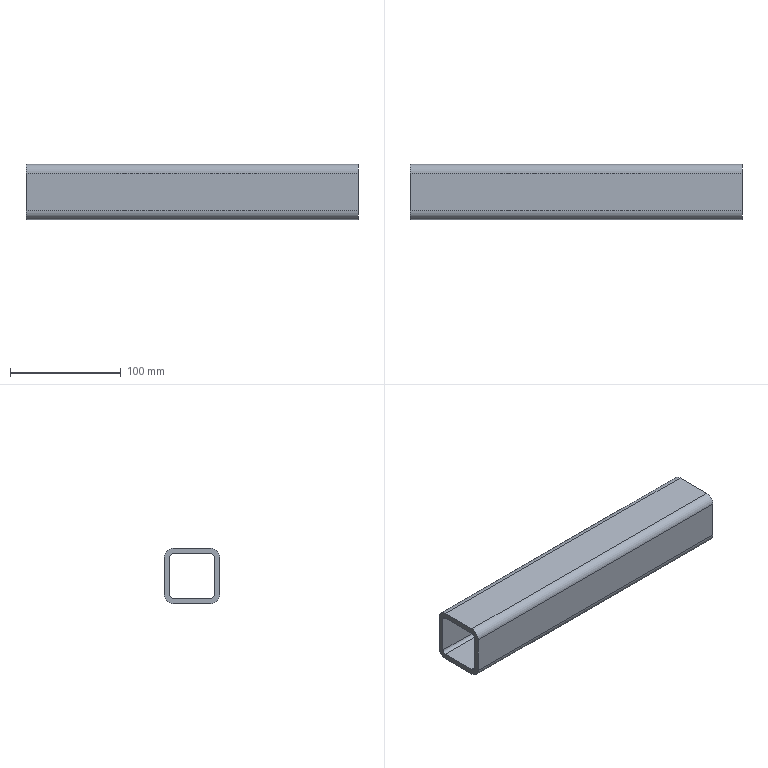Part | SolidWorks | features WeldMemberFeat 1, WeldmentFeature 1 | 1 solid | 18 faces | box 300 x 50 x 50 mm | volume 255836 mm3 | plane 10 | cylinder 8 | commonest cylinder face diameters 6 x4 16 x4
STEP:
#1=CARTESIAN_POINT('',(-88.434,25.,17.));
#2=VERTEX_POINT('',#1);
#3=CARTESIAN_POINT('',(-88.434,17.,25.));
#4=VERTEX_POINT('',#3);
#5=CARTESIAN_POINT('',(-88.434,17.,17.));
#6=DIRECTION('',(1.,0.,0.));
#7=DIRECTION('',(0.,0.,-1.));
#8=AXIS2_PLACEMENT_3D('',#5,#6,#7);
#9=CIRCLE('',#8,8.);
#10=EDGE_CURVE('',#2,#4,#9,.T.);
#11=ORIENTED_EDGE('',*,*,#10,.T.);
#12=CARTESIAN_POINT('',(211.566,17.,25.));
#13=VERTEX_POINT('',#12);
#14=CARTESIAN_POINT('',(211.566,17.,25.));
#15=DIRECTION('',(-1.,0.,0.));
#16=VECTOR('',#15,1000.);
#17=LINE('',#14,#16);
#18=EDGE_CURVE('',#13,#4,#17,.T.);
#19=ORIENTED_EDGE('',*,*,#18,.F.);
#20=CARTESIAN_POINT('',(211.566,25.,17.));
#21=VERTEX_POINT('',#20);
#22=CARTESIAN_POINT('',(211.566,17.,17.));
#23=DIRECTION('',(1.,0.,0.));
#24=DIRECTION('',(0.,0.,-1.));
#25=AXIS2_PLACEMENT_3D('',#22,#23,#24);
#26=CIRCLE('',#25,8.);
#27=EDGE_CURVE('',#21,#13,#26,.T.);
#28=ORIENTED_EDGE('',*,*,#27,.F.);
#29=CARTESIAN_POINT('',(211.566,25.,17.));
#30=DIRECTION('',(-1.,0.,0.));
#31=VECTOR('',#30,1000.);
#32=LINE('',#29,#31);
#33=EDGE_CURVE('',#21,#2,#32,.T.);
#34=ORIENTED_EDGE('',*,*,#33,.T.);
#35=EDGE_LOOP('',(#11,#19,#28,#34));
#36=FACE_OUTER_BOUND('',#35,.T.);
#37=CARTESIAN_POINT('',(211.566,17.,17.));
#38=DIRECTION('',(-1.,0.,0.));
#39=DIRECTION('',(0.,0.,1.));
#40=AXIS2_PLACEMENT_3D('',#37,#38,#39);
#41=CYLINDRICAL_SURFACE('',#40,8.);
#42=ADVANCED_FACE('',(#36),#41,.T.);
#43=CARTESIAN_POINT('',(-88.434,-17.,25.));
#44=VERTEX_POINT('',#43);
#45=CARTESIAN_POINT('',(-88.434,17.,25.));
#46=DIRECTION('',(0.,-1.,0.));
#47=VECTOR('',#46,1000.);
#48=LINE('',#45,#47);
#49=EDGE_CURVE('',#4,#44,#48,.T.);
#50=ORIENTED_EDGE('',*,*,#49,.T.);
#51=CARTESIAN_POINT('',(211.566,-17.,25.));
#52=VERTEX_POINT('',#51);
#53=CARTESIAN_POINT('',(211.566,-17.,25.));
#54=DIRECTION('',(-1.,0.,0.));
#55=VECTOR('',#54,1000.);
#56=LINE('',#53,#55);
#57=EDGE_CURVE('',#52,#44,#56,.T.);
#58=ORIENTED_EDGE('',*,*,#57,.F.);
#59=CARTESIAN_POINT('',(211.566,17.,25.));
#60=DIRECTION('',(0.,-1.,0.));
#61=VECTOR('',#60,1000.);
#62=LINE('',#59,#61);
#63=EDGE_CURVE('',#13,#52,#62,.T.);
#64=ORIENTED_EDGE('',*,*,#63,.F.);
#65=ORIENTED_EDGE('',*,*,#18,.T.);
#66=EDGE_LOOP('',(#50,#58,#64,#65));
#67=FACE_OUTER_BOUND('',#66,.T.);
#68=CARTESIAN_POINT('',(211.566,17.,25.));
#69=DIRECTION('',(0.,0.,-1.));
#70=DIRECTION('',(-1.,0.,0.));
#71=AXIS2_PLACEMENT_3D('',#68,#69,#70);
#72=PLANE('',#71);
#73=ADVANCED_FACE('',(#67),#72,.F.);
#74=CARTESIAN_POINT('',(-88.434,-25.,17.));
#75=VERTEX_POINT('',#74);
#76=CARTESIAN_POINT('',(-88.434,-17.,17.));
#77=DIRECTION('',(1.,0.,0.));
#78=DIRECTION('',(0.,0.,-1.));
#79=AXIS2_PLACEMENT_3D('',#76,#77,#78);
#80=CIRCLE('',#79,8.);
#81=EDGE_CURVE('',#44,#75,#80,.T.);
#82=ORIENTED_EDGE('',*,*,#81,.T.);
#83=CARTESIAN_POINT('',(211.566,-25.,17.));
#84=VERTEX_POINT('',#83);
#85=CARTESIAN_POINT('',(211.566,-25.,17.));
#86=DIRECTION('',(-1.,0.,0.));
#87=VECTOR('',#86,1000.);
#88=LINE('',#85,#87);
#89=EDGE_CURVE('',#84,#75,#88,.T.);
#90=ORIENTED_EDGE('',*,*,#89,.F.);
#91=CARTESIAN_POINT('',(211.566,-17.,17.));
#92=DIRECTION('',(1.,0.,0.));
#93=DIRECTION('',(0.,0.,-1.));
#94=AXIS2_PLACEMENT_3D('',#91,#92,#93);
#95=CIRCLE('',#94,8.);
#96=EDGE_CURVE('',#52,#84,#95,.T.);
#97=ORIENTED_EDGE('',*,*,#96,.F.);
#98=ORIENTED_EDGE('',*,*,#57,.T.);
#99=EDGE_LOOP('',(#82,#90,#97,#98));
#100=FACE_OUTER_BOUND('',#99,.T.);
#101=CARTESIAN_POINT('',(211.566,-17.,17.));
#102=DIRECTION('',(-1.,0.,0.));
#103=DIRECTION('',(0.,0.,1.));
#104=AXIS2_PLACEMENT_3D('',#101,#102,#103);
#105=CYLINDRICAL_SURFACE('',#104,8.);
#106=ADVANCED_FACE('',(#100),#105,.T.);
#107=CARTESIAN_POINT('',(-88.434,-25.,-17.));
#108=VERTEX_POINT('',#107);
#109=CARTESIAN_POINT('',(-88.434,-25.,-17.));
#110=DIRECTION('',(0.,0.,-1.));
#111=VECTOR('',#110,1000.);
#112=LINE('',#109,#111);
#113=EDGE_CURVE('',#75,#108,#112,.T.);
#114=ORIENTED_EDGE('',*,*,#113,.T.);
#115=CARTESIAN_POINT('',(211.566,-25.,-17.));
#116=VERTEX_POINT('',#115);
#117=CARTESIAN_POINT('',(211.566,-25.,-17.));
#118=DIRECTION('',(-1.,0.,0.));
#119=VECTOR('',#118,1000.);
#120=LINE('',#117,#119);
#121=EDGE_CURVE('',#116,#108,#120,.T.);
#122=ORIENTED_EDGE('',*,*,#121,.F.);
#123=CARTESIAN_POINT('',(211.566,-25.,-17.));
#124=DIRECTION('',(0.,0.,-1.));
#125=VECTOR('',#124,1000.);
#126=LINE('',#123,#125);
#127=EDGE_CURVE('',#84,#116,#126,.T.);
#128=ORIENTED_EDGE('',*,*,#127,.F.);
#129=ORIENTED_EDGE('',*,*,#89,.T.);
#130=EDGE_LOOP('',(#114,#122,#128,#129));
#131=FACE_OUTER_BOUND('',#130,.T.);
#132=CARTESIAN_POINT('',(211.566,-25.,-17.));
#133=DIRECTION('',(0.,1.,0.));
#134=DIRECTION('',(0.,0.,1.));
#135=AXIS2_PLACEMENT_3D('',#132,#133,#134);
#136=PLANE('',#135);
#137=ADVANCED_FACE('',(#131),#136,.F.);
#138=CARTESIAN_POINT('',(-88.434,-17.,-25.));
#139=VERTEX_POINT('',#138);
#140=CARTESIAN_POINT('',(-88.434,-17.,-17.));
#141=DIRECTION('',(1.,0.,0.));
#142=DIRECTION('',(0.,0.,-1.));
#143=AXIS2_PLACEMENT_3D('',#140,#141,#142);
#144=CIRCLE('',#143,8.);
#145=EDGE_CURVE('',#108,#139,#144,.T.);
#146=ORIENTED_EDGE('',*,*,#145,.T.);
#147=CARTESIAN_POINT('',(211.566,-17.,-25.));
#148=VERTEX_POINT('',#147);
#149=CARTESIAN_POINT('',(211.566,-17.,-25.));
#150=DIRECTION('',(-1.,0.,0.));
#151=VECTOR('',#150,1000.);
#152=LINE('',#149,#151);
#153=EDGE_CURVE('',#148,#139,#152,.T.);
#154=ORIENTED_EDGE('',*,*,#153,.F.);
#155=CARTESIAN_POINT('',(211.566,-17.,-17.));
#156=DIRECTION('',(1.,0.,0.));
#157=DIRECTION('',(0.,0.,-1.));
#158=AXIS2_PLACEMENT_3D('',#155,#156,#157);
#159=CIRCLE('',#158,8.);
#160=EDGE_CURVE('',#116,#148,#159,.T.);
#161=ORIENTED_EDGE('',*,*,#160,.F.);
#162=ORIENTED_EDGE('',*,*,#121,.T.);
#163=EDGE_LOOP('',(#146,#154,#161,#162));
#164=FACE_OUTER_BOUND('',#163,.T.);
#165=CARTESIAN_POINT('',(211.566,-17.,-17.));
#166=DIRECTION('',(-1.,0.,0.));
#167=DIRECTION('',(0.,0.,1.));
#168=AXIS2_PLACEMENT_3D('',#165,#166,#167);
#169=CYLINDRICAL_SURFACE('',#168,8.);
#170=ADVANCED_FACE('',(#164),#169,.T.);
#171=CARTESIAN_POINT('',(-88.434,17.,-25.));
#172=VERTEX_POINT('',#171);
#173=CARTESIAN_POINT('',(-88.434,-17.,-25.));
#174=DIRECTION('',(0.,1.,0.));
#175=VECTOR('',#174,1000.);
#176=LINE('',#173,#175);
#177=EDGE_CURVE('',#139,#172,#176,.T.);
#178=ORIENTED_EDGE('',*,*,#177,.T.);
#179=CARTESIAN_POINT('',(211.566,17.,-25.));
#180=VERTEX_POINT('',#179);
#181=CARTESIAN_POINT('',(211.566,17.,-25.));
#182=DIRECTION('',(-1.,0.,0.));
#183=VECTOR('',#182,1000.);
#184=LINE('',#181,#183);
#185=EDGE_CURVE('',#180,#172,#184,.T.);
#186=ORIENTED_EDGE('',*,*,#185,.F.);
#187=CARTESIAN_POINT('',(211.566,-17.,-25.));
#188=DIRECTION('',(0.,1.,0.));
#189=VECTOR('',#188,1000.);
#190=LINE('',#187,#189);
#191=EDGE_CURVE('',#148,#180,#190,.T.);
#192=ORIENTED_EDGE('',*,*,#191,.F.);
#193=ORIENTED_EDGE('',*,*,#153,.T.);
#194=EDGE_LOOP('',(#178,#186,#192,#193));
#195=FACE_OUTER_BOUND('',#194,.T.);
#196=CARTESIAN_POINT('',(211.566,-17.,-25.));
#197=DIRECTION('',(0.,0.,1.));
#198=DIRECTION('',(1.,0.,0.));
#199=AXIS2_PLACEMENT_3D('',#196,#197,#198);
#200=PLANE('',#199);
#201=ADVANCED_FACE('',(#195),#200,.F.);
#202=CARTESIAN_POINT('',(-88.434,25.,-17.));
#203=VERTEX_POINT('',#202);
#204=CARTESIAN_POINT('',(-88.434,17.,-17.));
#205=DIRECTION('',(1.,0.,0.));
#206=DIRECTION('',(0.,0.,-1.));
#207=AXIS2_PLACEMENT_3D('',#204,#205,#206);
#208=CIRCLE('',#207,8.);
#209=EDGE_CURVE('',#172,#203,#208,.T.);
#210=ORIENTED_EDGE('',*,*,#209,.T.);
#211=CARTESIAN_POINT('',(211.566,25.,-17.));
#212=VERTEX_POINT('',#211);
#213=CARTESIAN_POINT('',(211.566,25.,-17.));
#214=DIRECTION('',(-1.,0.,0.));
#215=VECTOR('',#214,1000.);
#216=LINE('',#213,#215);
#217=EDGE_CURVE('',#212,#203,#216,.T.);
#218=ORIENTED_EDGE('',*,*,#217,.F.);
#219=CARTESIAN_POINT('',(211.566,17.,-17.));
#220=DIRECTION('',(1.,0.,0.));
#221=DIRECTION('',(0.,0.,-1.));
#222=AXIS2_PLACEMENT_3D('',#219,#220,#221);
#223=CIRCLE('',#222,8.);
#224=EDGE_CURVE('',#180,#212,#223,.T.);
#225=ORIENTED_EDGE('',*,*,#224,.F.);
#226=ORIENTED_EDGE('',*,*,#185,.T.);
#227=EDGE_LOOP('',(#210,#218,#225,#226));
#228=FACE_OUTER_BOUND('',#227,.T.);
#229=CARTESIAN_POINT('',(211.566,17.,-17.));
#230=DIRECTION('',(-1.,0.,0.));
#231=DIRECTION('',(0.,0.,1.));
#232=AXIS2_PLACEMENT_3D('',#229,#230,#231);
#233=CYLINDRICAL_SURFACE('',#232,8.);
#234=ADVANCED_FACE('',(#228),#233,.T.);
#235=CARTESIAN_POINT('',(-88.434,-17.,20.));
#236=VERTEX_POINT('',#235);
#237=CARTESIAN_POINT('',(-88.434,-20.,17.));
#238=VERTEX_POINT('',#237);
#239=CARTESIAN_POINT('',(-88.434,-17.,17.));
#240=DIRECTION('',(1.,0.,0.));
#241=DIRECTION('',(0.,0.,-1.));
#242=AXIS2_PLACEMENT_3D('',#239,#240,#241);
#243=CIRCLE('',#242,3.);
#244=EDGE_CURVE('',#236,#238,#243,.T.);
#245=ORIENTED_EDGE('',*,*,#244,.F.);
#246=CARTESIAN_POINT('',(211.566,-17.,20.));
#247=VERTEX_POINT('',#246);
#248=CARTESIAN_POINT('',(211.566,-17.,20.));
#249=DIRECTION('',(-1.,0.,0.));
#250=VECTOR('',#249,1000.);
#251=LINE('',#248,#250);
#252=EDGE_CURVE('',#247,#236,#251,.T.);
#253=ORIENTED_EDGE('',*,*,#252,.F.);
#254=CARTESIAN_POINT('',(211.566,-20.,17.));
#255=VERTEX_POINT('',#254);
#256=CARTESIAN_POINT('',(211.566,-17.,17.));
#257=DIRECTION('',(1.,0.,0.));
#258=DIRECTION('',(0.,0.,-1.));
#259=AXIS2_PLACEMENT_3D('',#256,#257,#258);
#260=CIRCLE('',#259,3.);
#261=EDGE_CURVE('',#247,#255,#260,.T.);
#262=ORIENTED_EDGE('',*,*,#261,.T.);
#263=CARTESIAN_POINT('',(211.566,-20.,17.));
#264=DIRECTION('',(-1.,0.,0.));
#265=VECTOR('',#264,1000.);
#266=LINE('',#263,#265);
#267=EDGE_CURVE('',#255,#238,#266,.T.);
#268=ORIENTED_EDGE('',*,*,#267,.T.);
#269=EDGE_LOOP('',(#245,#253,#262,#268));
#270=FACE_OUTER_BOUND('',#269,.T.);
#271=CARTESIAN_POINT('',(211.566,-17.,17.));
#272=DIRECTION('',(-1.,0.,0.));
#273=DIRECTION('',(0.,0.,1.));
#274=AXIS2_PLACEMENT_3D('',#271,#272,#273);
#275=CYLINDRICAL_SURFACE('',#274,3.);
#276=ADVANCED_FACE('',(#270),#275,.F.);
#277=CARTESIAN_POINT('',(-88.434,17.,20.));
#278=VERTEX_POINT('',#277);
#279=CARTESIAN_POINT('',(-88.434,17.,20.));
#280=DIRECTION('',(0.,-1.,0.));
#281=VECTOR('',#280,1000.);
#282=LINE('',#279,#281);
#283=EDGE_CURVE('',#278,#236,#282,.T.);
#284=ORIENTED_EDGE('',*,*,#283,.F.);
#285=CARTESIAN_POINT('',(211.566,17.,20.));
#286=VERTEX_POINT('',#285);
#287=CARTESIAN_POINT('',(211.566,17.,20.));
#288=DIRECTION('',(-1.,0.,0.));
#289=VECTOR('',#288,1000.);
#290=LINE('',#287,#289);
#291=EDGE_CURVE('',#286,#278,#290,.T.);
#292=ORIENTED_EDGE('',*,*,#291,.F.);
#293=CARTESIAN_POINT('',(211.566,17.,20.));
#294=DIRECTION('',(0.,-1.,0.));
#295=VECTOR('',#294,1000.);
#296=LINE('',#293,#295);
#297=EDGE_CURVE('',#286,#247,#296,.T.);
#298=ORIENTED_EDGE('',*,*,#297,.T.);
#299=ORIENTED_EDGE('',*,*,#252,.T.);
#300=EDGE_LOOP('',(#284,#292,#298,#299));
#301=FACE_OUTER_BOUND('',#300,.T.);
#302=CARTESIAN_POINT('',(211.566,17.,20.));
#303=DIRECTION('',(0.,0.,-1.));
#304=DIRECTION('',(-1.,0.,0.));
#305=AXIS2_PLACEMENT_3D('',#302,#303,#304);
#306=PLANE('',#305);
#307=ADVANCED_FACE('',(#301),#306,.T.);
#308=CARTESIAN_POINT('',(-88.434,20.,17.));
#309=VERTEX_POINT('',#308);
#310=CARTESIAN_POINT('',(-88.434,17.,17.));
#311=DIRECTION('',(1.,0.,0.));
#312=DIRECTION('',(0.,0.,-1.));
#313=AXIS2_PLACEMENT_3D('',#310,#311,#312);
#314=CIRCLE('',#313,3.);
#315=EDGE_CURVE('',#309,#278,#314,.T.);
#316=ORIENTED_EDGE('',*,*,#315,.F.);
#317=CARTESIAN_POINT('',(211.566,20.,17.));
#318=VERTEX_POINT('',#317);
#319=CARTESIAN_POINT('',(211.566,20.,17.));
#320=DIRECTION('',(-1.,0.,0.));
#321=VECTOR('',#320,1000.);
#322=LINE('',#319,#321);
#323=EDGE_CURVE('',#318,#309,#322,.T.);
#324=ORIENTED_EDGE('',*,*,#323,.F.);
#325=CARTESIAN_POINT('',(211.566,17.,17.));
#326=DIRECTION('',(1.,0.,0.));
#327=DIRECTION('',(0.,0.,-1.));
#328=AXIS2_PLACEMENT_3D('',#325,#326,#327);
#329=CIRCLE('',#328,3.);
#330=EDGE_CURVE('',#318,#286,#329,.T.);
#331=ORIENTED_EDGE('',*,*,#330,.T.);
#332=ORIENTED_EDGE('',*,*,#291,.T.);
#333=EDGE_LOOP('',(#316,#324,#331,#332));
#334=FACE_OUTER_BOUND('',#333,.T.);
#335=CARTESIAN_POINT('',(211.566,17.,17.));
#336=DIRECTION('',(-1.,0.,0.));
#337=DIRECTION('',(0.,0.,1.));
#338=AXIS2_PLACEMENT_3D('',#335,#336,#337);
#339=CYLINDRICAL_SURFACE('',#338,3.);
#340=ADVANCED_FACE('',(#334),#339,.F.);
#341=CARTESIAN_POINT('',(-88.434,20.,-17.));
#342=VERTEX_POINT('',#341);
#343=CARTESIAN_POINT('',(-88.434,20.,17.));
#344=DIRECTION('',(0.,0.,1.));
#345=VECTOR('',#344,1000.);
#346=LINE('',#343,#345);
#347=EDGE_CURVE('',#342,#309,#346,.T.);
#348=ORIENTED_EDGE('',*,*,#347,.F.);
#349=CARTESIAN_POINT('',(211.566,20.,-17.));
#350=VERTEX_POINT('',#349);
#351=CARTESIAN_POINT('',(211.566,20.,-17.));
#352=DIRECTION('',(-1.,0.,0.));
#353=VECTOR('',#352,1000.);
#354=LINE('',#351,#353);
#355=EDGE_CURVE('',#350,#342,#354,.T.);
#356=ORIENTED_EDGE('',*,*,#355,.F.);
#357=CARTESIAN_POINT('',(211.566,20.,17.));
#358=DIRECTION('',(0.,0.,1.));
#359=VECTOR('',#358,1000.);
#360=LINE('',#357,#359);
#361=EDGE_CURVE('',#350,#318,#360,.T.);
#362=ORIENTED_EDGE('',*,*,#361,.T.);
#363=ORIENTED_EDGE('',*,*,#323,.T.);
#364=EDGE_LOOP('',(#348,#356,#362,#363));
#365=FACE_OUTER_BOUND('',#364,.T.);
#366=CARTESIAN_POINT('',(211.566,20.,17.));
#367=DIRECTION('',(0.,-1.,0.));
#368=DIRECTION('',(0.,0.,-1.));
#369=AXIS2_PLACEMENT_3D('',#366,#367,#368);
#370=PLANE('',#369);
#371=ADVANCED_FACE('',(#365),#370,.T.);
#372=CARTESIAN_POINT('',(-88.434,17.,-20.));
#373=VERTEX_POINT('',#372);
#374=CARTESIAN_POINT('',(-88.434,17.,-17.));
#375=DIRECTION('',(1.,0.,0.));
#376=DIRECTION('',(0.,0.,-1.));
#377=AXIS2_PLACEMENT_3D('',#374,#375,#376);
#378=CIRCLE('',#377,3.);
#379=EDGE_CURVE('',#373,#342,#378,.T.);
#380=ORIENTED_EDGE('',*,*,#379,.F.);
#381=CARTESIAN_POINT('',(211.566,17.,-20.));
#382=VERTEX_POINT('',#381);
#383=CARTESIAN_POINT('',(211.566,17.,-20.));
#384=DIRECTION('',(-1.,0.,0.));
#385=VECTOR('',#384,1000.);
#386=LINE('',#383,#385);
#387=EDGE_CURVE('',#382,#373,#386,.T.);
#388=ORIENTED_EDGE('',*,*,#387,.F.);
#389=CARTESIAN_POINT('',(211.566,17.,-17.));
#390=DIRECTION('',(1.,0.,0.));
#391=DIRECTION('',(0.,0.,-1.));
#392=AXIS2_PLACEMENT_3D('',#389,#390,#391);
#393=CIRCLE('',#392,3.);
#394=EDGE_CURVE('',#382,#350,#393,.T.);
#395=ORIENTED_EDGE('',*,*,#394,.T.);
#396=ORIENTED_EDGE('',*,*,#355,.T.);
#397=EDGE_LOOP('',(#380,#388,#395,#396));
#398=FACE_OUTER_BOUND('',#397,.T.);
#399=CARTESIAN_POINT('',(211.566,17.,-17.));
#400=DIRECTION('',(-1.,0.,0.));
#401=DIRECTION('',(0.,0.,1.));
#402=AXIS2_PLACEMENT_3D('',#399,#400,#401);
#403=CYLINDRICAL_SURFACE('',#402,3.);
#404=ADVANCED_FACE('',(#398),#403,.F.);
#405=CARTESIAN_POINT('',(-88.434,-17.,-20.));
#406=VERTEX_POINT('',#405);
#407=CARTESIAN_POINT('',(-88.434,-17.,-20.));
#408=DIRECTION('',(0.,1.,0.));
#409=VECTOR('',#408,1000.);
#410=LINE('',#407,#409);
#411=EDGE_CURVE('',#406,#373,#410,.T.);
#412=ORIENTED_EDGE('',*,*,#411,.F.);
#413=CARTESIAN_POINT('',(211.566,-17.,-20.));
#414=VERTEX_POINT('',#413);
#415=CARTESIAN_POINT('',(211.566,-17.,-20.));
#416=DIRECTION('',(-1.,0.,0.));
#417=VECTOR('',#416,1000.);
#418=LINE('',#415,#417);
#419=EDGE_CURVE('',#414,#406,#418,.T.);
#420=ORIENTED_EDGE('',*,*,#419,.F.);
#421=CARTESIAN_POINT('',(211.566,-17.,-20.));
#422=DIRECTION('',(0.,1.,0.));
#423=VECTOR('',#422,1000.);
#424=LINE('',#421,#423);
#425=EDGE_CURVE('',#414,#382,#424,.T.);
#426=ORIENTED_EDGE('',*,*,#425,.T.);
#427=ORIENTED_EDGE('',*,*,#387,.T.);
#428=EDGE_LOOP('',(#412,#420,#426,#427));
#429=FACE_OUTER_BOUND('',#428,.T.);
#430=CARTESIAN_POINT('',(211.566,-17.,-20.));
#431=DIRECTION('',(0.,0.,1.));
#432=DIRECTION('',(1.,0.,0.));
#433=AXIS2_PLACEMENT_3D('',#430,#431,#432);
#434=PLANE('',#433);
#435=ADVANCED_FACE('',(#429),#434,.T.);
#436=CARTESIAN_POINT('',(-88.434,-20.,-17.));
#437=VERTEX_POINT('',#436);
#438=CARTESIAN_POINT('',(-88.434,-17.,-17.));
#439=DIRECTION('',(1.,0.,0.));
#440=DIRECTION('',(0.,0.,-1.));
#441=AXIS2_PLACEMENT_3D('',#438,#439,#440);
#442=CIRCLE('',#441,3.);
#443=EDGE_CURVE('',#437,#406,#442,.T.);
#444=ORIENTED_EDGE('',*,*,#443,.F.);
#445=CARTESIAN_POINT('',(211.566,-20.,-17.));
#446=VERTEX_POINT('',#445);
#447=CARTESIAN_POINT('',(211.566,-20.,-17.));
#448=DIRECTION('',(-1.,0.,0.));
#449=VECTOR('',#448,1000.);
#450=LINE('',#447,#449);
#451=EDGE_CURVE('',#446,#437,#450,.T.);
#452=ORIENTED_EDGE('',*,*,#451,.F.);
#453=CARTESIAN_POINT('',(211.566,-17.,-17.));
#454=DIRECTION('',(1.,0.,0.));
#455=DIRECTION('',(0.,0.,-1.));
#456=AXIS2_PLACEMENT_3D('',#453,#454,#455);
#457=CIRCLE('',#456,3.);
#458=EDGE_CURVE('',#446,#414,#457,.T.);
#459=ORIENTED_EDGE('',*,*,#458,.T.);
#460=ORIENTED_EDGE('',*,*,#419,.T.);
#461=EDGE_LOOP('',(#444,#452,#459,#460));
#462=FACE_OUTER_BOUND('',#461,.T.);
#463=CARTESIAN_POINT('',(211.566,-17.,-17.));
#464=DIRECTION('',(-1.,0.,0.));
#465=DIRECTION('',(0.,0.,1.));
#466=AXIS2_PLACEMENT_3D('',#463,#464,#465);
#467=CYLINDRICAL_SURFACE('',#466,3.);
#468=ADVANCED_FACE('',(#462),#467,.F.);
#469=CARTESIAN_POINT('',(-88.434,-20.,-17.));
#470=DIRECTION('',(0.,0.,-1.));
#471=VECTOR('',#470,1000.);
#472=LINE('',#469,#471);
#473=EDGE_CURVE('',#238,#437,#472,.T.);
#474=ORIENTED_EDGE('',*,*,#473,.F.);
#475=ORIENTED_EDGE('',*,*,#267,.F.);
#476=CARTESIAN_POINT('',(211.566,-20.,-17.));
#477=DIRECTION('',(0.,0.,-1.));
#478=VECTOR('',#477,1000.);
#479=LINE('',#476,#478);
#480=EDGE_CURVE('',#255,#446,#479,.T.);
#481=ORIENTED_EDGE('',*,*,#480,.T.);
#482=ORIENTED_EDGE('',*,*,#451,.T.);
#483=EDGE_LOOP('',(#474,#475,#481,#482));
#484=FACE_OUTER_BOUND('',#483,.T.);
#485=CARTESIAN_POINT('',(211.566,-20.,-17.));
#486=DIRECTION('',(0.,1.,0.));
#487=DIRECTION('',(0.,0.,1.));
#488=AXIS2_PLACEMENT_3D('',#485,#486,#487);
#489=PLANE('',#488);
#490=ADVANCED_FACE('',(#484),#489,.T.);
#491=CARTESIAN_POINT('',(-88.434,25.,17.));
#492=DIRECTION('',(0.,0.,1.));
#493=VECTOR('',#492,1000.);
#494=LINE('',#491,#493);
#495=EDGE_CURVE('',#203,#2,#494,.T.);
#496=ORIENTED_EDGE('',*,*,#495,.T.);
#497=ORIENTED_EDGE('',*,*,#33,.F.);
#498=CARTESIAN_POINT('',(211.566,25.,17.));
#499=DIRECTION('',(0.,0.,1.));
#500=VECTOR('',#499,1000.);
#501=LINE('',#498,#500);
#502=EDGE_CURVE('',#212,#21,#501,.T.);
#503=ORIENTED_EDGE('',*,*,#502,.F.);
#504=ORIENTED_EDGE('',*,*,#217,.T.);
#505=EDGE_LOOP('',(#496,#497,#503,#504));
#506=FACE_OUTER_BOUND('',#505,.T.);
#507=CARTESIAN_POINT('',(211.566,25.,17.));
#508=DIRECTION('',(0.,-1.,0.));
#509=DIRECTION('',(0.,0.,-1.));
#510=AXIS2_PLACEMENT_3D('',#507,#508,#509);
#511=PLANE('',#510);
#512=ADVANCED_FACE('',(#506),#511,.F.);
#513=ORIENTED_EDGE('',*,*,#261,.F.);
#514=ORIENTED_EDGE('',*,*,#297,.F.);
#515=ORIENTED_EDGE('',*,*,#330,.F.);
#516=ORIENTED_EDGE('',*,*,#361,.F.);
#517=ORIENTED_EDGE('',*,*,#394,.F.);
#518=ORIENTED_EDGE('',*,*,#425,.F.);
#519=ORIENTED_EDGE('',*,*,#458,.F.);
#520=ORIENTED_EDGE('',*,*,#480,.F.);
#521=EDGE_LOOP('',(#513,#514,#515,#516,#517,#518,#519,#520));
#522=FACE_BOUND('',#521,.T.);
#523=ORIENTED_EDGE('',*,*,#27,.T.);
#524=ORIENTED_EDGE('',*,*,#63,.T.);
#525=ORIENTED_EDGE('',*,*,#96,.T.);
#526=ORIENTED_EDGE('',*,*,#127,.T.);
#527=ORIENTED_EDGE('',*,*,#160,.T.);
#528=ORIENTED_EDGE('',*,*,#191,.T.);
#529=ORIENTED_EDGE('',*,*,#224,.T.);
#530=ORIENTED_EDGE('',*,*,#502,.T.);
#531=EDGE_LOOP('',(#523,#524,#525,#526,#527,#528,#529,#530));
#532=FACE_OUTER_BOUND('',#531,.T.);
#533=CARTESIAN_POINT('',(211.566,17.,17.));
#534=DIRECTION('',(1.,0.,0.));
#535=DIRECTION('',(0.,0.,-1.));
#536=AXIS2_PLACEMENT_3D('',#533,#534,#535);
#537=PLANE('',#536);
#538=ADVANCED_FACE('',(#522,#532),#537,.T.);
#539=ORIENTED_EDGE('',*,*,#244,.T.);
#540=ORIENTED_EDGE('',*,*,#473,.T.);
#541=ORIENTED_EDGE('',*,*,#443,.T.);
#542=ORIENTED_EDGE('',*,*,#411,.T.);
#543=ORIENTED_EDGE('',*,*,#379,.T.);
#544=ORIENTED_EDGE('',*,*,#347,.T.);
#545=ORIENTED_EDGE('',*,*,#315,.T.);
#546=ORIENTED_EDGE('',*,*,#283,.T.);
#547=EDGE_LOOP('',(#539,#540,#541,#542,#543,#544,#545,#546));
#548=FACE_BOUND('',#547,.T.);
#549=ORIENTED_EDGE('',*,*,#10,.F.);
#550=ORIENTED_EDGE('',*,*,#495,.F.);
#551=ORIENTED_EDGE('',*,*,#209,.F.);
#552=ORIENTED_EDGE('',*,*,#177,.F.);
#553=ORIENTED_EDGE('',*,*,#145,.F.);
#554=ORIENTED_EDGE('',*,*,#113,.F.);
#555=ORIENTED_EDGE('',*,*,#81,.F.);
#556=ORIENTED_EDGE('',*,*,#49,.F.);
#557=EDGE_LOOP('',(#549,#550,#551,#552,#553,#554,#555,#556));
#558=FACE_OUTER_BOUND('',#557,.T.);
#559=CARTESIAN_POINT('',(-88.434,17.,17.));
#560=DIRECTION('',(1.,0.,0.));
#561=DIRECTION('',(0.,0.,-1.));
#562=AXIS2_PLACEMENT_3D('',#559,#560,#561);
#563=PLANE('',#562);
#564=ADVANCED_FACE('',(#548,#558),#563,.F.);
#565=CLOSED_SHELL('',(#42,#73,#106,#137,#170,#201,#234,#276,#307,#340,#371,#404,#435,#468,#490,#512,#538,#564));
#566=MANIFOLD_SOLID_BREP('',#565);
#567=CARTESIAN_POINT('',(0.,0.,0.));
#568=DIRECTION('',(0.,0.,1.));
#569=DIRECTION('',(1.,0.,0.));
#570=AXIS2_PLACEMENT_3D('',#567,#568,#569);
#571=(LENGTH_UNIT()NAMED_UNIT(*)SI_UNIT(.MILLI.,.METRE.));
#572=UNCERTAINTY_MEASURE_WITH_UNIT(LENGTH_MEASURE(0.00001),#571,'','');
#573=(NAMED_UNIT(*)PLANE_ANGLE_UNIT()SI_UNIT($,.RADIAN.));
#574=(NAMED_UNIT(*)SI_UNIT($,.STERADIAN.)SOLID_ANGLE_UNIT());
#575=(GEOMETRIC_REPRESENTATION_CONTEXT(3)GLOBAL_UNCERTAINTY_ASSIGNED_CONTEXT((#572))GLOBAL_UNIT_ASSIGNED_CONTEXT((#571,#573,#574))REPRESENTATION_CONTEXT('',''));
#576=ADVANCED_BREP_SHAPE_REPRESENTATION('',(#566,#570),#575);